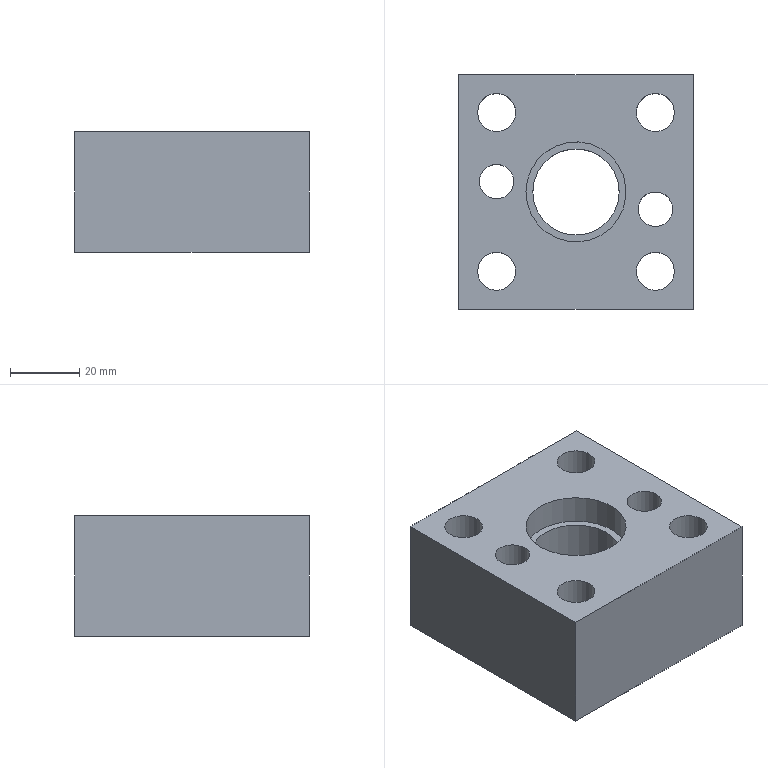Part | NX | features solid 2 | 1 solid | 27 faces | box 68 x 68 x 35 mm | volume 117785 mm3 | cylinder 14 | plane 13 | commonest cylinder face diameters 11 x6 17 x4 10 x2 25 x1 29 x1
STEP:
#1=CARTESIAN_POINT('',(1105.579,-146.904,53.));
#2=VERTEX_POINT('',#1);
#3=CARTESIAN_POINT('',(1111.079,-146.904,53.));
#4=DIRECTION('',(0.,0.,-1.));
#5=DIRECTION('',(-1.,0.,0.));
#6=AXIS2_PLACEMENT_3D('',#3,#4,#5);
#7=CIRCLE('',#6,5.5);
#8=EDGE_CURVE('',#2,#2,#7,.T.);
#9=ORIENTED_EDGE('',*,*,#8,.F.);
#10=EDGE_LOOP('',(#9));
#11=FACE_BOUND('',#10,.T.);
#12=CARTESIAN_POINT('',(1105.579,-146.904,43.));
#13=VERTEX_POINT('',#12);
#14=CARTESIAN_POINT('',(1111.079,-146.904,43.));
#15=DIRECTION('',(0.,0.,-1.));
#16=DIRECTION('',(-1.,0.,0.));
#17=AXIS2_PLACEMENT_3D('',#14,#15,#16);
#18=CIRCLE('',#17,5.5);
#19=EDGE_CURVE('',#13,#13,#18,.F.);
#20=ORIENTED_EDGE('',*,*,#19,.F.);
#21=EDGE_LOOP('',(#20));
#22=FACE_BOUND('',#21,.T.);
#23=CARTESIAN_POINT('',(1111.079,-146.904,43.));
#24=DIRECTION('',(0.,0.,1.));
#25=DIRECTION('',(-1.,0.,0.));
#26=AXIS2_PLACEMENT_3D('',#23,#24,#25);
#27=CYLINDRICAL_SURFACE('',#26,5.5);
#28=ADVANCED_FACE('',(#11,#22),#27,.F.);
#29=CARTESIAN_POINT('',(1116.079,-146.904,53.));
#30=VERTEX_POINT('',#29);
#31=CARTESIAN_POINT('',(1111.079,-146.904,53.));
#32=DIRECTION('',(0.,0.,1.));
#33=DIRECTION('',(1.,0.,0.));
#34=AXIS2_PLACEMENT_3D('',#31,#32,#33);
#35=CIRCLE('',#34,5.);
#36=EDGE_CURVE('',#30,#30,#35,.F.);
#37=ORIENTED_EDGE('',*,*,#36,.F.);
#38=EDGE_LOOP('',(#37));
#39=FACE_BOUND('',#38,.T.);
#40=ORIENTED_EDGE('',*,*,#8,.T.);
#41=EDGE_LOOP('',(#40));
#42=FACE_BOUND('',#41,.T.);
#43=CARTESIAN_POINT('',(1112.263,-137.78,53.));
#44=DIRECTION('',(0.,0.,1.));
#45=DIRECTION('',(-1.,0.,0.));
#46=AXIS2_PLACEMENT_3D('',#43,#44,#45);
#47=PLANE('',#46);
#48=ADVANCED_FACE('',(#39,#42),#47,.F.);
#49=CARTESIAN_POINT('',(1106.079,-146.904,78.));
#50=VERTEX_POINT('',#49);
#51=CARTESIAN_POINT('',(1111.079,-146.904,78.));
#52=DIRECTION('',(0.,0.,-1.));
#53=DIRECTION('',(-1.,0.,0.));
#54=AXIS2_PLACEMENT_3D('',#51,#52,#53);
#55=CIRCLE('',#54,5.);
#56=EDGE_CURVE('',#50,#50,#55,.T.);
#57=ORIENTED_EDGE('',*,*,#56,.F.);
#58=EDGE_LOOP('',(#57));
#59=FACE_BOUND('',#58,.T.);
#60=ORIENTED_EDGE('',*,*,#36,.T.);
#61=EDGE_LOOP('',(#60));
#62=FACE_BOUND('',#61,.T.);
#63=CARTESIAN_POINT('',(1111.079,-146.904,78.));
#64=DIRECTION('',(0.,0.,1.));
#65=DIRECTION('',(-1.,0.,0.));
#66=AXIS2_PLACEMENT_3D('',#63,#64,#65);
#67=CYLINDRICAL_SURFACE('',#66,5.);
#68=ADVANCED_FACE('',(#59,#62),#67,.F.);
#69=CARTESIAN_POINT('',(1070.579,-118.904,55.));
#70=VERTEX_POINT('',#69);
#71=CARTESIAN_POINT('',(1065.079,-118.904,55.));
#72=DIRECTION('',(0.,0.,1.));
#73=DIRECTION('',(1.,0.,0.));
#74=AXIS2_PLACEMENT_3D('',#71,#72,#73);
#75=CIRCLE('',#74,5.5);
#76=EDGE_CURVE('',#70,#70,#75,.F.);
#77=ORIENTED_EDGE('',*,*,#76,.F.);
#78=EDGE_LOOP('',(#77));
#79=FACE_BOUND('',#78,.T.);
#80=CARTESIAN_POINT('',(1073.579,-118.904,55.));
#81=VERTEX_POINT('',#80);
#82=CARTESIAN_POINT('',(1065.079,-118.904,55.));
#83=DIRECTION('',(0.,0.,1.));
#84=DIRECTION('',(1.,0.,0.));
#85=AXIS2_PLACEMENT_3D('',#82,#83,#84);
#86=CIRCLE('',#85,8.5);
#87=EDGE_CURVE('',#81,#81,#86,.F.);
#88=ORIENTED_EDGE('',*,*,#87,.T.);
#89=EDGE_LOOP('',(#88));
#90=FACE_BOUND('',#89,.T.);
#91=CARTESIAN_POINT('',(1065.083,-120.57,55.));
#92=DIRECTION('',(0.,0.,1.));
#93=DIRECTION('',(1.,0.,0.));
#94=AXIS2_PLACEMENT_3D('',#91,#92,#93);
#95=PLANE('',#94);
#96=ADVANCED_FACE('',(#79,#90),#95,.F.);
#97=CARTESIAN_POINT('',(1070.579,-164.904,55.));
#98=VERTEX_POINT('',#97);
#99=CARTESIAN_POINT('',(1065.079,-164.904,55.));
#100=DIRECTION('',(0.,0.,-1.));
#101=DIRECTION('',(1.,0.,0.));
#102=AXIS2_PLACEMENT_3D('',#99,#100,#101);
#103=CIRCLE('',#102,5.5);
#104=EDGE_CURVE('',#98,#98,#103,.T.);
#105=ORIENTED_EDGE('',*,*,#104,.F.);
#106=EDGE_LOOP('',(#105));
#107=FACE_BOUND('',#106,.T.);
#108=CARTESIAN_POINT('',(1073.579,-164.904,55.));
#109=VERTEX_POINT('',#108);
#110=CARTESIAN_POINT('',(1065.079,-164.904,55.));
#111=DIRECTION('',(0.,0.,-1.));
#112=DIRECTION('',(1.,0.,0.));
#113=AXIS2_PLACEMENT_3D('',#110,#111,#112);
#114=CIRCLE('',#113,8.5);
#115=EDGE_CURVE('',#109,#109,#114,.T.);
#116=ORIENTED_EDGE('',*,*,#115,.T.);
#117=EDGE_LOOP('',(#116));
#118=FACE_BOUND('',#117,.T.);
#119=CARTESIAN_POINT('',(1065.083,-163.238,55.));
#120=DIRECTION('',(0.,0.,1.));
#121=DIRECTION('',(1.,0.,0.));
#122=AXIS2_PLACEMENT_3D('',#119,#120,#121);
#123=PLANE('',#122);
#124=ADVANCED_FACE('',(#107,#118),#123,.F.);
#125=CARTESIAN_POINT('',(1105.579,-164.904,55.));
#126=VERTEX_POINT('',#125);
#127=CARTESIAN_POINT('',(1111.079,-164.904,55.));
#128=DIRECTION('',(0.,0.,1.));
#129=DIRECTION('',(-1.,0.,0.));
#130=AXIS2_PLACEMENT_3D('',#127,#128,#129);
#131=CIRCLE('',#130,5.5);
#132=EDGE_CURVE('',#126,#126,#131,.F.);
#133=ORIENTED_EDGE('',*,*,#132,.F.);
#134=EDGE_LOOP('',(#133));
#135=FACE_BOUND('',#134,.T.);
#136=CARTESIAN_POINT('',(1102.579,-164.904,55.));
#137=VERTEX_POINT('',#136);
#138=CARTESIAN_POINT('',(1111.079,-164.904,55.));
#139=DIRECTION('',(0.,0.,1.));
#140=DIRECTION('',(-1.,0.,0.));
#141=AXIS2_PLACEMENT_3D('',#138,#139,#140);
#142=CIRCLE('',#141,8.5);
#143=EDGE_CURVE('',#137,#137,#142,.F.);
#144=ORIENTED_EDGE('',*,*,#143,.T.);
#145=EDGE_LOOP('',(#144));
#146=FACE_BOUND('',#145,.T.);
#147=CARTESIAN_POINT('',(1111.074,-163.238,55.));
#148=DIRECTION('',(0.,0.,1.));
#149=DIRECTION('',(-1.,0.,0.));
#150=AXIS2_PLACEMENT_3D('',#147,#148,#149);
#151=PLANE('',#150);
#152=ADVANCED_FACE('',(#135,#146),#151,.F.);
#153=CARTESIAN_POINT('',(1105.579,-118.904,55.));
#154=VERTEX_POINT('',#153);
#155=CARTESIAN_POINT('',(1111.079,-118.904,55.));
#156=DIRECTION('',(0.,0.,-1.));
#157=DIRECTION('',(-1.,0.,0.));
#158=AXIS2_PLACEMENT_3D('',#155,#156,#157);
#159=CIRCLE('',#158,5.5);
#160=EDGE_CURVE('',#154,#154,#159,.T.);
#161=ORIENTED_EDGE('',*,*,#160,.F.);
#162=EDGE_LOOP('',(#161));
#163=FACE_BOUND('',#162,.T.);
#164=CARTESIAN_POINT('',(1102.579,-118.904,55.));
#165=VERTEX_POINT('',#164);
#166=CARTESIAN_POINT('',(1111.079,-118.904,55.));
#167=DIRECTION('',(0.,0.,-1.));
#168=DIRECTION('',(-1.,0.,0.));
#169=AXIS2_PLACEMENT_3D('',#166,#167,#168);
#170=CIRCLE('',#169,8.5);
#171=EDGE_CURVE('',#165,#165,#170,.T.);
#172=ORIENTED_EDGE('',*,*,#171,.T.);
#173=EDGE_LOOP('',(#172));
#174=FACE_BOUND('',#173,.T.);
#175=CARTESIAN_POINT('',(1111.074,-120.57,55.));
#176=DIRECTION('',(0.,0.,1.));
#177=DIRECTION('',(-1.,0.,0.));
#178=AXIS2_PLACEMENT_3D('',#175,#176,#177);
#179=PLANE('',#178);
#180=ADVANCED_FACE('',(#163,#174),#179,.F.);
#181=CARTESIAN_POINT('',(1070.079,-138.904,53.));
#182=VERTEX_POINT('',#181);
#183=CARTESIAN_POINT('',(1065.079,-138.904,53.));
#184=DIRECTION('',(0.,0.,1.));
#185=DIRECTION('',(1.,0.,0.));
#186=AXIS2_PLACEMENT_3D('',#183,#184,#185);
#187=CIRCLE('',#186,5.);
#188=EDGE_CURVE('',#182,#182,#187,.F.);
#189=ORIENTED_EDGE('',*,*,#188,.F.);
#190=EDGE_LOOP('',(#189));
#191=FACE_BOUND('',#190,.T.);
#192=CARTESIAN_POINT('',(1070.579,-138.904,53.));
#193=VERTEX_POINT('',#192);
#194=CARTESIAN_POINT('',(1065.079,-138.904,53.));
#195=DIRECTION('',(0.,0.,1.));
#196=DIRECTION('',(1.,0.,0.));
#197=AXIS2_PLACEMENT_3D('',#194,#195,#196);
#198=CIRCLE('',#197,5.5);
#199=EDGE_CURVE('',#193,#193,#198,.F.);
#200=ORIENTED_EDGE('',*,*,#199,.T.);
#201=EDGE_LOOP('',(#200));
#202=FACE_BOUND('',#201,.T.);
#203=CARTESIAN_POINT('',(1063.894,-137.78,53.));
#204=DIRECTION('',(0.,0.,1.));
#205=DIRECTION('',(1.,0.,0.));
#206=AXIS2_PLACEMENT_3D('',#203,#204,#205);
#207=PLANE('',#206);
#208=ADVANCED_FACE('',(#191,#202),#207,.F.);
#209=CARTESIAN_POINT('',(1054.079,-175.904,43.));
#210=VERTEX_POINT('',#209);
#211=CARTESIAN_POINT('',(1054.079,-175.904,78.));
#212=VERTEX_POINT('',#211);
#213=CARTESIAN_POINT('',(1054.079,-175.904,50.));
#214=DIRECTION('',(0.,0.,1.));
#215=VECTOR('',#214,1000.);
#216=LINE('',#213,#215);
#217=EDGE_CURVE('',#210,#212,#216,.T.);
#218=ORIENTED_EDGE('',*,*,#217,.T.);
#219=CARTESIAN_POINT('',(1054.079,-107.904,78.));
#220=VERTEX_POINT('',#219);
#221=CARTESIAN_POINT('',(1054.079,-141.904,78.));
#222=DIRECTION('',(0.,-1.,0.));
#223=VECTOR('',#222,1000.);
#224=LINE('',#221,#223);
#225=EDGE_CURVE('',#212,#220,#224,.F.);
#226=ORIENTED_EDGE('',*,*,#225,.T.);
#227=CARTESIAN_POINT('',(1054.079,-107.904,43.));
#228=VERTEX_POINT('',#227);
#229=CARTESIAN_POINT('',(1054.079,-107.904,50.));
#230=DIRECTION('',(0.,0.,1.));
#231=VECTOR('',#230,1000.);
#232=LINE('',#229,#231);
#233=EDGE_CURVE('',#228,#220,#232,.T.);
#234=ORIENTED_EDGE('',*,*,#233,.F.);
#235=CARTESIAN_POINT('',(1054.079,-141.904,43.));
#236=DIRECTION('',(0.,-1.,0.));
#237=VECTOR('',#236,1000.);
#238=LINE('',#235,#237);
#239=EDGE_CURVE('',#228,#210,#238,.T.);
#240=ORIENTED_EDGE('',*,*,#239,.T.);
#241=EDGE_LOOP('',(#218,#226,#234,#240));
#242=FACE_BOUND('',#241,.T.);
#243=CARTESIAN_POINT('',(1054.079,-141.904,50.));
#244=DIRECTION('',(-1.,0.,0.));
#245=DIRECTION('',(0.,0.,1.));
#246=AXIS2_PLACEMENT_3D('',#243,#244,#245);
#247=PLANE('',#246);
#248=ADVANCED_FACE('',(#242),#247,.T.);
#249=ORIENTED_EDGE('',*,*,#233,.T.);
#250=CARTESIAN_POINT('',(1122.079,-107.904,78.));
#251=VERTEX_POINT('',#250);
#252=CARTESIAN_POINT('',(1088.079,-107.904,78.));
#253=DIRECTION('',(-1.,0.,0.));
#254=VECTOR('',#253,1000.);
#255=LINE('',#252,#254);
#256=EDGE_CURVE('',#220,#251,#255,.F.);
#257=ORIENTED_EDGE('',*,*,#256,.T.);
#258=CARTESIAN_POINT('',(1122.079,-107.904,43.));
#259=VERTEX_POINT('',#258);
#260=CARTESIAN_POINT('',(1122.079,-107.904,50.));
#261=DIRECTION('',(0.,0.,1.));
#262=VECTOR('',#261,1000.);
#263=LINE('',#260,#262);
#264=EDGE_CURVE('',#259,#251,#263,.T.);
#265=ORIENTED_EDGE('',*,*,#264,.F.);
#266=CARTESIAN_POINT('',(1088.079,-107.904,43.));
#267=DIRECTION('',(-1.,0.,0.));
#268=VECTOR('',#267,1000.);
#269=LINE('',#266,#268);
#270=EDGE_CURVE('',#259,#228,#269,.T.);
#271=ORIENTED_EDGE('',*,*,#270,.T.);
#272=EDGE_LOOP('',(#249,#257,#265,#271));
#273=FACE_BOUND('',#272,.T.);
#274=CARTESIAN_POINT('',(1088.079,-107.904,50.));
#275=DIRECTION('',(0.,1.,0.));
#276=DIRECTION('',(0.,0.,1.));
#277=AXIS2_PLACEMENT_3D('',#274,#275,#276);
#278=PLANE('',#277);
#279=ADVANCED_FACE('',(#273),#278,.T.);
#280=CARTESIAN_POINT('',(1122.079,-175.904,43.));
#281=VERTEX_POINT('',#280);
#282=CARTESIAN_POINT('',(1122.079,-141.904,43.));
#283=DIRECTION('',(0.,1.,0.));
#284=VECTOR('',#283,1000.);
#285=LINE('',#282,#284);
#286=EDGE_CURVE('',#281,#259,#285,.T.);
#287=ORIENTED_EDGE('',*,*,#286,.T.);
#288=ORIENTED_EDGE('',*,*,#264,.T.);
#289=CARTESIAN_POINT('',(1122.079,-175.904,78.));
#290=VERTEX_POINT('',#289);
#291=CARTESIAN_POINT('',(1122.079,-141.904,78.));
#292=DIRECTION('',(0.,1.,0.));
#293=VECTOR('',#292,1000.);
#294=LINE('',#291,#293);
#295=EDGE_CURVE('',#251,#290,#294,.F.);
#296=ORIENTED_EDGE('',*,*,#295,.T.);
#297=CARTESIAN_POINT('',(1122.079,-175.904,50.));
#298=DIRECTION('',(0.,0.,1.));
#299=VECTOR('',#298,1000.);
#300=LINE('',#297,#299);
#301=EDGE_CURVE('',#281,#290,#300,.T.);
#302=ORIENTED_EDGE('',*,*,#301,.F.);
#303=EDGE_LOOP('',(#287,#288,#296,#302));
#304=FACE_BOUND('',#303,.T.);
#305=CARTESIAN_POINT('',(1122.079,-141.904,50.));
#306=DIRECTION('',(1.,0.,0.));
#307=DIRECTION('',(0.,0.,-1.));
#308=AXIS2_PLACEMENT_3D('',#305,#306,#307);
#309=PLANE('',#308);
#310=ADVANCED_FACE('',(#304),#309,.T.);
#311=ORIENTED_EDGE('',*,*,#301,.T.);
#312=CARTESIAN_POINT('',(1088.079,-175.904,78.));
#313=DIRECTION('',(1.,0.,0.));
#314=VECTOR('',#313,1000.);
#315=LINE('',#312,#314);
#316=EDGE_CURVE('',#290,#212,#315,.F.);
#317=ORIENTED_EDGE('',*,*,#316,.T.);
#318=ORIENTED_EDGE('',*,*,#217,.F.);
#319=CARTESIAN_POINT('',(1088.079,-175.904,43.));
#320=DIRECTION('',(1.,0.,0.));
#321=VECTOR('',#320,1000.);
#322=LINE('',#319,#321);
#323=EDGE_CURVE('',#210,#281,#322,.T.);
#324=ORIENTED_EDGE('',*,*,#323,.T.);
#325=EDGE_LOOP('',(#311,#317,#318,#324));
#326=FACE_BOUND('',#325,.T.);
#327=CARTESIAN_POINT('',(1088.079,-175.904,50.));
#328=DIRECTION('',(0.,-1.,0.));
#329=DIRECTION('',(0.,0.,-1.));
#330=AXIS2_PLACEMENT_3D('',#327,#328,#329);
#331=PLANE('',#330);
#332=ADVANCED_FACE('',(#326),#331,.T.);
#333=CARTESIAN_POINT('',(1070.579,-118.904,78.));
#334=VERTEX_POINT('',#333);
#335=CARTESIAN_POINT('',(1065.079,-118.904,78.));
#336=DIRECTION('',(0.,0.,1.));
#337=DIRECTION('',(1.,0.,0.));
#338=AXIS2_PLACEMENT_3D('',#335,#336,#337);
#339=CIRCLE('',#338,5.5);
#340=EDGE_CURVE('',#334,#334,#339,.T.);
#341=ORIENTED_EDGE('',*,*,#340,.T.);
#342=EDGE_LOOP('',(#341));
#343=FACE_BOUND('',#342,.T.);
#344=ORIENTED_EDGE('',*,*,#76,.T.);
#345=EDGE_LOOP('',(#344));
#346=FACE_BOUND('',#345,.T.);
#347=CARTESIAN_POINT('',(1065.079,-118.904,78.));
#348=DIRECTION('',(0.,0.,1.));
#349=DIRECTION('',(1.,0.,0.));
#350=AXIS2_PLACEMENT_3D('',#347,#348,#349);
#351=CYLINDRICAL_SURFACE('',#350,5.5);
#352=ADVANCED_FACE('',(#343,#346),#351,.F.);
#353=CARTESIAN_POINT('',(1070.579,-164.904,78.));
#354=VERTEX_POINT('',#353);
#355=CARTESIAN_POINT('',(1065.079,-164.904,78.));
#356=DIRECTION('',(0.,0.,-1.));
#357=DIRECTION('',(1.,0.,0.));
#358=AXIS2_PLACEMENT_3D('',#355,#356,#357);
#359=CIRCLE('',#358,5.5);
#360=EDGE_CURVE('',#354,#354,#359,.T.);
#361=ORIENTED_EDGE('',*,*,#360,.F.);
#362=EDGE_LOOP('',(#361));
#363=FACE_BOUND('',#362,.T.);
#364=ORIENTED_EDGE('',*,*,#104,.T.);
#365=EDGE_LOOP('',(#364));
#366=FACE_BOUND('',#365,.T.);
#367=CARTESIAN_POINT('',(1065.079,-164.904,78.));
#368=DIRECTION('',(0.,0.,1.));
#369=DIRECTION('',(1.,0.,0.));
#370=AXIS2_PLACEMENT_3D('',#367,#368,#369);
#371=CYLINDRICAL_SURFACE('',#370,5.5);
#372=ADVANCED_FACE('',(#363,#366),#371,.F.);
#373=CARTESIAN_POINT('',(1105.579,-164.904,78.));
#374=VERTEX_POINT('',#373);
#375=CARTESIAN_POINT('',(1111.079,-164.904,78.));
#376=DIRECTION('',(0.,0.,1.));
#377=DIRECTION('',(-1.,0.,0.));
#378=AXIS2_PLACEMENT_3D('',#375,#376,#377);
#379=CIRCLE('',#378,5.5);
#380=EDGE_CURVE('',#374,#374,#379,.F.);
#381=ORIENTED_EDGE('',*,*,#380,.F.);
#382=EDGE_LOOP('',(#381));
#383=FACE_BOUND('',#382,.T.);
#384=ORIENTED_EDGE('',*,*,#132,.T.);
#385=EDGE_LOOP('',(#384));
#386=FACE_BOUND('',#385,.T.);
#387=CARTESIAN_POINT('',(1111.079,-164.904,78.));
#388=DIRECTION('',(0.,0.,1.));
#389=DIRECTION('',(-1.,0.,0.));
#390=AXIS2_PLACEMENT_3D('',#387,#388,#389);
#391=CYLINDRICAL_SURFACE('',#390,5.5);
#392=ADVANCED_FACE('',(#383,#386),#391,.F.);
#393=CARTESIAN_POINT('',(1105.579,-118.904,78.));
#394=VERTEX_POINT('',#393);
#395=CARTESIAN_POINT('',(1111.079,-118.904,78.));
#396=DIRECTION('',(0.,0.,-1.));
#397=DIRECTION('',(-1.,0.,0.));
#398=AXIS2_PLACEMENT_3D('',#395,#396,#397);
#399=CIRCLE('',#398,5.5);
#400=EDGE_CURVE('',#394,#394,#399,.T.);
#401=ORIENTED_EDGE('',*,*,#400,.F.);
#402=EDGE_LOOP('',(#401));
#403=FACE_BOUND('',#402,.T.);
#404=ORIENTED_EDGE('',*,*,#160,.T.);
#405=EDGE_LOOP('',(#404));
#406=FACE_BOUND('',#405,.T.);
#407=CARTESIAN_POINT('',(1111.079,-118.904,78.));
#408=DIRECTION('',(0.,0.,1.));
#409=DIRECTION('',(-1.,0.,0.));
#410=AXIS2_PLACEMENT_3D('',#407,#408,#409);
#411=CYLINDRICAL_SURFACE('',#410,5.5);
#412=ADVANCED_FACE('',(#403,#406),#411,.F.);
#413=CARTESIAN_POINT('',(1060.079,-138.904,78.));
#414=VERTEX_POINT('',#413);
#415=CARTESIAN_POINT('',(1065.079,-138.904,78.));
#416=DIRECTION('',(0.,0.,-1.));
#417=DIRECTION('',(-1.,0.,0.));
#418=AXIS2_PLACEMENT_3D('',#415,#416,#417);
#419=CIRCLE('',#418,5.);
#420=EDGE_CURVE('',#414,#414,#419,.F.);
#421=ORIENTED_EDGE('',*,*,#420,.T.);
#422=EDGE_LOOP('',(#421));
#423=FACE_BOUND('',#422,.T.);
#424=ORIENTED_EDGE('',*,*,#188,.T.);
#425=EDGE_LOOP('',(#424));
#426=FACE_BOUND('',#425,.T.);
#427=CARTESIAN_POINT('',(1065.079,-138.904,78.));
#428=DIRECTION('',(0.,0.,1.));
#429=DIRECTION('',(1.,0.,0.));
#430=AXIS2_PLACEMENT_3D('',#427,#428,#429);
#431=CYLINDRICAL_SURFACE('',#430,5.);
#432=ADVANCED_FACE('',(#423,#426),#431,.F.);
#433=CARTESIAN_POINT('',(1073.579,-141.904,78.));
#434=VERTEX_POINT('',#433);
#435=CARTESIAN_POINT('',(1088.079,-141.904,78.));
#436=DIRECTION('',(0.,0.,-1.));
#437=DIRECTION('',(-1.,0.,0.));
#438=AXIS2_PLACEMENT_3D('',#435,#436,#437);
#439=CIRCLE('',#438,14.5);
#440=EDGE_CURVE('',#434,#434,#439,.T.);
#441=ORIENTED_EDGE('',*,*,#440,.T.);
#442=EDGE_LOOP('',(#441));
#443=FACE_BOUND('',#442,.T.);
#444=ORIENTED_EDGE('',*,*,#56,.T.);
#445=EDGE_LOOP('',(#444));
#446=FACE_BOUND('',#445,.T.);
#447=ORIENTED_EDGE('',*,*,#420,.F.);
#448=EDGE_LOOP('',(#447));
#449=FACE_BOUND('',#448,.T.);
#450=ORIENTED_EDGE('',*,*,#400,.T.);
#451=EDGE_LOOP('',(#450));
#452=FACE_BOUND('',#451,.T.);
#453=ORIENTED_EDGE('',*,*,#380,.T.);
#454=EDGE_LOOP('',(#453));
#455=FACE_BOUND('',#454,.T.);
#456=ORIENTED_EDGE('',*,*,#360,.T.);
#457=EDGE_LOOP('',(#456));
#458=FACE_BOUND('',#457,.T.);
#459=ORIENTED_EDGE('',*,*,#340,.F.);
#460=EDGE_LOOP('',(#459));
#461=FACE_BOUND('',#460,.T.);
#462=ORIENTED_EDGE('',*,*,#316,.F.);
#463=ORIENTED_EDGE('',*,*,#295,.F.);
#464=ORIENTED_EDGE('',*,*,#256,.F.);
#465=ORIENTED_EDGE('',*,*,#225,.F.);
#466=EDGE_LOOP('',(#462,#463,#464,#465));
#467=FACE_BOUND('',#466,.T.);
#468=CARTESIAN_POINT('',(287.,-0.000000688,78.));
#469=DIRECTION('',(0.,0.,-1.));
#470=DIRECTION('',(-1.,0.,0.));
#471=AXIS2_PLACEMENT_3D('',#468,#469,#470);
#472=PLANE('',#471);
#473=ADVANCED_FACE('',(#443,#446,#449,#452,#455,#458,#461,#467),#472,.F.);
#474=ORIENTED_EDGE('',*,*,#87,.F.);
#475=EDGE_LOOP('',(#474));
#476=FACE_BOUND('',#475,.T.);
#477=CARTESIAN_POINT('',(1073.579,-118.904,43.));
#478=VERTEX_POINT('',#477);
#479=CARTESIAN_POINT('',(1065.079,-118.904,43.));
#480=DIRECTION('',(0.,0.,1.));
#481=DIRECTION('',(1.,0.,0.));
#482=AXIS2_PLACEMENT_3D('',#479,#480,#481);
#483=CIRCLE('',#482,8.5);
#484=EDGE_CURVE('',#478,#478,#483,.T.);
#485=ORIENTED_EDGE('',*,*,#484,.F.);
#486=EDGE_LOOP('',(#485));
#487=FACE_BOUND('',#486,.T.);
#488=CARTESIAN_POINT('',(1065.079,-118.904,43.));
#489=DIRECTION('',(0.,0.,1.));
#490=DIRECTION('',(1.,0.,0.));
#491=AXIS2_PLACEMENT_3D('',#488,#489,#490);
#492=CYLINDRICAL_SURFACE('',#491,8.5);
#493=ADVANCED_FACE('',(#476,#487),#492,.F.);
#494=ORIENTED_EDGE('',*,*,#115,.F.);
#495=EDGE_LOOP('',(#494));
#496=FACE_BOUND('',#495,.T.);
#497=CARTESIAN_POINT('',(1073.579,-164.904,43.));
#498=VERTEX_POINT('',#497);
#499=CARTESIAN_POINT('',(1065.079,-164.904,43.));
#500=DIRECTION('',(0.,0.,-1.));
#501=DIRECTION('',(1.,0.,0.));
#502=AXIS2_PLACEMENT_3D('',#499,#500,#501);
#503=CIRCLE('',#502,8.5);
#504=EDGE_CURVE('',#498,#498,#503,.F.);
#505=ORIENTED_EDGE('',*,*,#504,.F.);
#506=EDGE_LOOP('',(#505));
#507=FACE_BOUND('',#506,.T.);
#508=CARTESIAN_POINT('',(1065.079,-164.904,43.));
#509=DIRECTION('',(0.,0.,1.));
#510=DIRECTION('',(1.,0.,0.));
#511=AXIS2_PLACEMENT_3D('',#508,#509,#510);
#512=CYLINDRICAL_SURFACE('',#511,8.5);
#513=ADVANCED_FACE('',(#496,#507),#512,.F.);
#514=ORIENTED_EDGE('',*,*,#143,.F.);
#515=EDGE_LOOP('',(#514));
#516=FACE_BOUND('',#515,.T.);
#517=CARTESIAN_POINT('',(1102.579,-164.904,43.));
#518=VERTEX_POINT('',#517);
#519=CARTESIAN_POINT('',(1111.079,-164.904,43.));
#520=DIRECTION('',(0.,0.,1.));
#521=DIRECTION('',(-1.,0.,0.));
#522=AXIS2_PLACEMENT_3D('',#519,#520,#521);
#523=CIRCLE('',#522,8.5);
#524=EDGE_CURVE('',#518,#518,#523,.T.);
#525=ORIENTED_EDGE('',*,*,#524,.F.);
#526=EDGE_LOOP('',(#525));
#527=FACE_BOUND('',#526,.T.);
#528=CARTESIAN_POINT('',(1111.079,-164.904,43.));
#529=DIRECTION('',(0.,0.,1.));
#530=DIRECTION('',(-1.,0.,0.));
#531=AXIS2_PLACEMENT_3D('',#528,#529,#530);
#532=CYLINDRICAL_SURFACE('',#531,8.5);
#533=ADVANCED_FACE('',(#516,#527),#532,.F.);
#534=ORIENTED_EDGE('',*,*,#171,.F.);
#535=EDGE_LOOP('',(#534));
#536=FACE_BOUND('',#535,.T.);
#537=CARTESIAN_POINT('',(1102.579,-118.904,43.));
#538=VERTEX_POINT('',#537);
#539=CARTESIAN_POINT('',(1111.079,-118.904,43.));
#540=DIRECTION('',(0.,0.,-1.));
#541=DIRECTION('',(-1.,0.,0.));
#542=AXIS2_PLACEMENT_3D('',#539,#540,#541);
#543=CIRCLE('',#542,8.5);
#544=EDGE_CURVE('',#538,#538,#543,.F.);
#545=ORIENTED_EDGE('',*,*,#544,.F.);
#546=EDGE_LOOP('',(#545));
#547=FACE_BOUND('',#546,.T.);
#548=CARTESIAN_POINT('',(1111.079,-118.904,43.));
#549=DIRECTION('',(0.,0.,1.));
#550=DIRECTION('',(-1.,0.,0.));
#551=AXIS2_PLACEMENT_3D('',#548,#549,#550);
#552=CYLINDRICAL_SURFACE('',#551,8.5);
#553=ADVANCED_FACE('',(#536,#547),#552,.F.);
#554=ORIENTED_EDGE('',*,*,#199,.F.);
#555=EDGE_LOOP('',(#554));
#556=FACE_BOUND('',#555,.T.);
#557=CARTESIAN_POINT('',(1070.579,-138.904,43.));
#558=VERTEX_POINT('',#557);
#559=CARTESIAN_POINT('',(1065.079,-138.904,43.));
#560=DIRECTION('',(0.,0.,1.));
#561=DIRECTION('',(1.,0.,0.));
#562=AXIS2_PLACEMENT_3D('',#559,#560,#561);
#563=CIRCLE('',#562,5.5);
#564=EDGE_CURVE('',#558,#558,#563,.T.);
#565=ORIENTED_EDGE('',*,*,#564,.F.);
#566=EDGE_LOOP('',(#565));
#567=FACE_BOUND('',#566,.T.);
#568=CARTESIAN_POINT('',(1065.079,-138.904,43.));
#569=DIRECTION('',(0.,0.,1.));
#570=DIRECTION('',(1.,0.,0.));
#571=AXIS2_PLACEMENT_3D('',#568,#569,#570);
#572=CYLINDRICAL_SURFACE('',#571,5.5);
#573=ADVANCED_FACE('',(#556,#567),#572,.F.);
#574=CARTESIAN_POINT('',(1075.579,-141.904,43.));
#575=VERTEX_POINT('',#574);
#576=CARTESIAN_POINT('',(1088.079,-141.904,43.));
#577=DIRECTION('',(0.,0.,-1.));
#578=DIRECTION('',(-1.,0.,0.));
#579=AXIS2_PLACEMENT_3D('',#576,#577,#578);
#580=CIRCLE('',#579,12.5);
#581=EDGE_CURVE('',#575,#575,#580,.T.);
#582=ORIENTED_EDGE('',*,*,#581,.F.);
#583=EDGE_LOOP('',(#582));
#584=FACE_BOUND('',#583,.T.);
#585=ORIENTED_EDGE('',*,*,#19,.T.);
#586=EDGE_LOOP('',(#585));
#587=FACE_BOUND('',#586,.T.);
#588=ORIENTED_EDGE('',*,*,#564,.T.);
#589=EDGE_LOOP('',(#588));
#590=FACE_BOUND('',#589,.T.);
#591=ORIENTED_EDGE('',*,*,#544,.T.);
#592=EDGE_LOOP('',(#591));
#593=FACE_BOUND('',#592,.T.);
#594=ORIENTED_EDGE('',*,*,#524,.T.);
#595=EDGE_LOOP('',(#594));
#596=FACE_BOUND('',#595,.T.);
#597=ORIENTED_EDGE('',*,*,#504,.T.);
#598=EDGE_LOOP('',(#597));
#599=FACE_BOUND('',#598,.T.);
#600=ORIENTED_EDGE('',*,*,#484,.T.);
#601=EDGE_LOOP('',(#600));
#602=FACE_BOUND('',#601,.T.);
#603=ORIENTED_EDGE('',*,*,#286,.F.);
#604=ORIENTED_EDGE('',*,*,#323,.F.);
#605=ORIENTED_EDGE('',*,*,#239,.F.);
#606=ORIENTED_EDGE('',*,*,#270,.F.);
#607=EDGE_LOOP('',(#603,#604,#605,#606));
#608=FACE_BOUND('',#607,.T.);
#609=CARTESIAN_POINT('',(1088.079,-141.904,43.));
#610=DIRECTION('',(0.,0.,-1.));
#611=DIRECTION('',(-1.,0.,0.));
#612=AXIS2_PLACEMENT_3D('',#609,#610,#611);
#613=PLANE('',#612);
#614=ADVANCED_FACE('',(#584,#587,#590,#593,#596,#599,#602,#608),#613,.T.);
#615=ORIENTED_EDGE('',*,*,#581,.T.);
#616=EDGE_LOOP('',(#615));
#617=FACE_BOUND('',#616,.T.);
#618=CARTESIAN_POINT('',(1075.579,-141.904,69.7));
#619=VERTEX_POINT('',#618);
#620=CARTESIAN_POINT('',(1088.079,-141.904,69.7));
#621=DIRECTION('',(0.,0.,-1.));
#622=DIRECTION('',(-1.,0.,0.));
#623=AXIS2_PLACEMENT_3D('',#620,#621,#622);
#624=CIRCLE('',#623,12.5);
#625=EDGE_CURVE('',#619,#619,#624,.T.);
#626=ORIENTED_EDGE('',*,*,#625,.F.);
#627=EDGE_LOOP('',(#626));
#628=FACE_BOUND('',#627,.T.);
#629=CARTESIAN_POINT('',(1088.079,-141.904,78.));
#630=DIRECTION('',(0.,0.,-1.));
#631=DIRECTION('',(-1.,0.,0.));
#632=AXIS2_PLACEMENT_3D('',#629,#630,#631);
#633=CYLINDRICAL_SURFACE('',#632,12.5);
#634=ADVANCED_FACE('',(#617,#628),#633,.F.);
#635=ORIENTED_EDGE('',*,*,#440,.F.);
#636=EDGE_LOOP('',(#635));
#637=FACE_BOUND('',#636,.T.);
#638=CARTESIAN_POINT('',(1073.579,-141.904,69.7));
#639=VERTEX_POINT('',#638);
#640=CARTESIAN_POINT('',(1088.079,-141.904,69.7));
#641=DIRECTION('',(0.,0.,-1.));
#642=DIRECTION('',(-1.,0.,0.));
#643=AXIS2_PLACEMENT_3D('',#640,#641,#642);
#644=CIRCLE('',#643,14.5);
#645=EDGE_CURVE('',#639,#639,#644,.F.);
#646=ORIENTED_EDGE('',*,*,#645,.F.);
#647=EDGE_LOOP('',(#646));
#648=FACE_BOUND('',#647,.T.);
#649=CARTESIAN_POINT('',(1088.079,-141.904,78.));
#650=DIRECTION('',(0.,0.,-1.));
#651=DIRECTION('',(-1.,0.,0.));
#652=AXIS2_PLACEMENT_3D('',#649,#650,#651);
#653=CYLINDRICAL_SURFACE('',#652,14.5);
#654=ADVANCED_FACE('',(#637,#648),#653,.F.);
#655=ORIENTED_EDGE('',*,*,#625,.T.);
#656=EDGE_LOOP('',(#655));
#657=FACE_BOUND('',#656,.T.);
#658=ORIENTED_EDGE('',*,*,#645,.T.);
#659=EDGE_LOOP('',(#658));
#660=FACE_BOUND('',#659,.T.);
#661=CARTESIAN_POINT('',(1088.079,-141.904,69.7));
#662=DIRECTION('',(0.,0.,-1.));
#663=DIRECTION('',(-1.,0.,0.));
#664=AXIS2_PLACEMENT_3D('',#661,#662,#663);
#665=PLANE('',#664);
#666=ADVANCED_FACE('',(#657,#660),#665,.F.);
#667=CLOSED_SHELL('',(#28,#48,#68,#96,#124,#152,#180,#208,#248,#279,#310,#332,#352,#372,#392,#412,#432,#473,#493,#513,#533,#553,#573,#614,#634,#654,#666));
#668=MANIFOLD_SOLID_BREP('',#667);
#669=(LENGTH_UNIT()NAMED_UNIT(*)SI_UNIT(.MILLI.,.METRE.));
#670=UNCERTAINTY_MEASURE_WITH_UNIT(LENGTH_MEASURE(0.00001),#669,'','');
#671=(NAMED_UNIT(*)PLANE_ANGLE_UNIT()SI_UNIT($,.RADIAN.));
#672=(NAMED_UNIT(*)SI_UNIT($,.STERADIAN.)SOLID_ANGLE_UNIT());
#673=(GEOMETRIC_REPRESENTATION_CONTEXT(3)GLOBAL_UNCERTAINTY_ASSIGNED_CONTEXT((#670))GLOBAL_UNIT_ASSIGNED_CONTEXT((#669,#671,#672))REPRESENTATION_CONTEXT('',''));
#674=ADVANCED_BREP_SHAPE_REPRESENTATION('',(#668),#673);